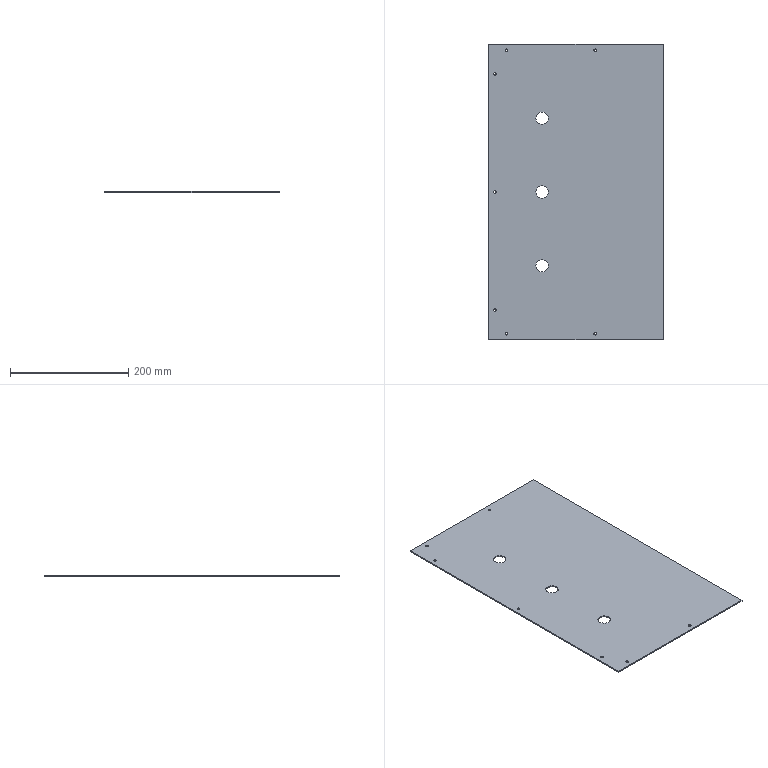Part | SolidWorks | features Extrusion 1, HoleWzd 1, ICE 1 | 1 solid | 26 faces | box 295 x 500 x 2 mm | volume 292699 mm3 | cylinder 20 | plane 6 | commonest cylinder face diameters 4.5 x14 21 x6
STEP:
#1=CARTESIAN_POINT('',(-68.,125.,0.));
#2=VERTEX_POINT('',#1);
#3=CARTESIAN_POINT('',(-47.,125.,0.));
#4=VERTEX_POINT('',#3);
#5=CARTESIAN_POINT('',(-57.5,125.,0.));
#6=DIRECTION('',(0.,0.,1.));
#7=DIRECTION('',(1.,0.,0.));
#8=AXIS2_PLACEMENT_3D('',#5,#6,#7);
#9=CIRCLE('',#8,10.5);
#10=EDGE_CURVE('',#2,#4,#9,.T.);
#11=ORIENTED_EDGE('',*,*,#10,.F.);
#12=CARTESIAN_POINT('',(-68.,125.,2.));
#13=VERTEX_POINT('',#12);
#14=CARTESIAN_POINT('',(-68.,125.,-8.));
#15=DIRECTION('',(0.,0.,1.));
#16=VECTOR('',#15,1000.);
#17=LINE('',#14,#16);
#18=EDGE_CURVE('',#2,#13,#17,.T.);
#19=ORIENTED_EDGE('',*,*,#18,.T.);
#20=CARTESIAN_POINT('',(-47.,125.,2.));
#21=VERTEX_POINT('',#20);
#22=CARTESIAN_POINT('',(-57.5,125.,2.));
#23=DIRECTION('',(0.,0.,1.));
#24=DIRECTION('',(1.,0.,0.));
#25=AXIS2_PLACEMENT_3D('',#22,#23,#24);
#26=CIRCLE('',#25,10.5);
#27=EDGE_CURVE('',#13,#21,#26,.T.);
#28=ORIENTED_EDGE('',*,*,#27,.T.);
#29=CARTESIAN_POINT('',(-47.,125.,-8.));
#30=DIRECTION('',(0.,0.,1.));
#31=VECTOR('',#30,1000.);
#32=LINE('',#29,#31);
#33=EDGE_CURVE('',#4,#21,#32,.T.);
#34=ORIENTED_EDGE('',*,*,#33,.F.);
#35=EDGE_LOOP('',(#11,#19,#28,#34));
#36=FACE_OUTER_BOUND('',#35,.T.);
#37=CARTESIAN_POINT('',(-57.5,125.,-8.));
#38=DIRECTION('',(0.,0.,1.));
#39=DIRECTION('',(1.,0.,0.));
#40=AXIS2_PLACEMENT_3D('',#37,#38,#39);
#41=CYLINDRICAL_SURFACE('',#40,10.5);
#42=ADVANCED_FACE('',(#36),#41,.F.);
#43=CARTESIAN_POINT('',(-68.,-125.,0.));
#44=VERTEX_POINT('',#43);
#45=CARTESIAN_POINT('',(-47.,-125.,0.));
#46=VERTEX_POINT('',#45);
#47=CARTESIAN_POINT('',(-57.5,-125.,0.));
#48=DIRECTION('',(0.,0.,1.));
#49=DIRECTION('',(1.,0.,0.));
#50=AXIS2_PLACEMENT_3D('',#47,#48,#49);
#51=CIRCLE('',#50,10.5);
#52=EDGE_CURVE('',#44,#46,#51,.T.);
#53=ORIENTED_EDGE('',*,*,#52,.F.);
#54=CARTESIAN_POINT('',(-68.,-125.,2.));
#55=VERTEX_POINT('',#54);
#56=CARTESIAN_POINT('',(-68.,-125.,-8.));
#57=DIRECTION('',(0.,0.,1.));
#58=VECTOR('',#57,1000.);
#59=LINE('',#56,#58);
#60=EDGE_CURVE('',#44,#55,#59,.T.);
#61=ORIENTED_EDGE('',*,*,#60,.T.);
#62=CARTESIAN_POINT('',(-47.,-125.,2.));
#63=VERTEX_POINT('',#62);
#64=CARTESIAN_POINT('',(-57.5,-125.,2.));
#65=DIRECTION('',(0.,0.,1.));
#66=DIRECTION('',(-1.,0.,0.));
#67=AXIS2_PLACEMENT_3D('',#64,#65,#66);
#68=CIRCLE('',#67,10.5);
#69=EDGE_CURVE('',#55,#63,#68,.T.);
#70=ORIENTED_EDGE('',*,*,#69,.T.);
#71=CARTESIAN_POINT('',(-47.,-125.,-8.));
#72=DIRECTION('',(0.,0.,1.));
#73=VECTOR('',#72,1000.);
#74=LINE('',#71,#73);
#75=EDGE_CURVE('',#46,#63,#74,.T.);
#76=ORIENTED_EDGE('',*,*,#75,.F.);
#77=EDGE_LOOP('',(#53,#61,#70,#76));
#78=FACE_OUTER_BOUND('',#77,.T.);
#79=CARTESIAN_POINT('',(-57.5,-125.,-8.));
#80=DIRECTION('',(0.,0.,1.));
#81=DIRECTION('',(1.,0.,0.));
#82=AXIS2_PLACEMENT_3D('',#79,#80,#81);
#83=CYLINDRICAL_SURFACE('',#82,10.5);
#84=ADVANCED_FACE('',(#78),#83,.F.);
#85=CARTESIAN_POINT('',(-68.,0.,0.));
#86=VERTEX_POINT('',#85);
#87=CARTESIAN_POINT('',(-47.,0.,0.));
#88=VERTEX_POINT('',#87);
#89=CARTESIAN_POINT('',(-57.5,0.,0.));
#90=DIRECTION('',(0.,0.,1.));
#91=DIRECTION('',(1.,0.,0.));
#92=AXIS2_PLACEMENT_3D('',#89,#90,#91);
#93=CIRCLE('',#92,10.5);
#94=EDGE_CURVE('',#86,#88,#93,.T.);
#95=ORIENTED_EDGE('',*,*,#94,.F.);
#96=CARTESIAN_POINT('',(-68.,0.,2.));
#97=VERTEX_POINT('',#96);
#98=CARTESIAN_POINT('',(-68.,0.,-8.));
#99=DIRECTION('',(0.,0.,1.));
#100=VECTOR('',#99,1000.);
#101=LINE('',#98,#100);
#102=EDGE_CURVE('',#86,#97,#101,.T.);
#103=ORIENTED_EDGE('',*,*,#102,.T.);
#104=CARTESIAN_POINT('',(-47.,0.,2.));
#105=VERTEX_POINT('',#104);
#106=CARTESIAN_POINT('',(-57.5,0.,2.));
#107=DIRECTION('',(0.,0.,1.));
#108=DIRECTION('',(1.,0.,0.));
#109=AXIS2_PLACEMENT_3D('',#106,#107,#108);
#110=CIRCLE('',#109,10.5);
#111=EDGE_CURVE('',#97,#105,#110,.T.);
#112=ORIENTED_EDGE('',*,*,#111,.T.);
#113=CARTESIAN_POINT('',(-47.,0.,-8.));
#114=DIRECTION('',(0.,0.,1.));
#115=VECTOR('',#114,1000.);
#116=LINE('',#113,#115);
#117=EDGE_CURVE('',#88,#105,#116,.T.);
#118=ORIENTED_EDGE('',*,*,#117,.F.);
#119=EDGE_LOOP('',(#95,#103,#112,#118));
#120=FACE_OUTER_BOUND('',#119,.T.);
#121=CARTESIAN_POINT('',(-57.5,0.,-8.));
#122=DIRECTION('',(0.,0.,1.));
#123=DIRECTION('',(1.,0.,0.));
#124=AXIS2_PLACEMENT_3D('',#121,#122,#123);
#125=CYLINDRICAL_SURFACE('',#124,10.5);
#126=ADVANCED_FACE('',(#120),#125,.F.);
#127=CARTESIAN_POINT('',(-139.75,0.,0.));
#128=VERTEX_POINT('',#127);
#129=CARTESIAN_POINT('',(-135.25,0.,0.));
#130=VERTEX_POINT('',#129);
#131=CARTESIAN_POINT('',(-137.5,0.,0.));
#132=DIRECTION('',(0.,0.,1.));
#133=DIRECTION('',(1.,0.,0.));
#134=AXIS2_PLACEMENT_3D('',#131,#132,#133);
#135=CIRCLE('',#134,2.25);
#136=EDGE_CURVE('',#128,#130,#135,.T.);
#137=ORIENTED_EDGE('',*,*,#136,.F.);
#138=CARTESIAN_POINT('',(-139.75,0.,2.));
#139=VERTEX_POINT('',#138);
#140=CARTESIAN_POINT('',(-139.75,0.,2.));
#141=DIRECTION('',(0.,0.,1.));
#142=VECTOR('',#141,1000.);
#143=LINE('',#140,#142);
#144=EDGE_CURVE('',#128,#139,#143,.T.);
#145=ORIENTED_EDGE('',*,*,#144,.T.);
#146=CARTESIAN_POINT('',(-135.25,0.,2.));
#147=VERTEX_POINT('',#146);
#148=CARTESIAN_POINT('',(-137.5,0.,2.));
#149=DIRECTION('',(0.,0.,1.));
#150=DIRECTION('',(1.,0.,0.));
#151=AXIS2_PLACEMENT_3D('',#148,#149,#150);
#152=CIRCLE('',#151,2.25);
#153=EDGE_CURVE('',#139,#147,#152,.T.);
#154=ORIENTED_EDGE('',*,*,#153,.T.);
#155=CARTESIAN_POINT('',(-135.25,0.,2.));
#156=DIRECTION('',(0.,0.,1.));
#157=VECTOR('',#156,1000.);
#158=LINE('',#155,#157);
#159=EDGE_CURVE('',#130,#147,#158,.T.);
#160=ORIENTED_EDGE('',*,*,#159,.F.);
#161=EDGE_LOOP('',(#137,#145,#154,#160));
#162=FACE_OUTER_BOUND('',#161,.T.);
#163=CARTESIAN_POINT('',(-137.5,0.,2.));
#164=DIRECTION('',(0.,0.,1.));
#165=DIRECTION('',(1.,0.,0.));
#166=AXIS2_PLACEMENT_3D('',#163,#164,#165);
#167=CYLINDRICAL_SURFACE('',#166,2.25);
#168=ADVANCED_FACE('',(#162),#167,.F.);
#169=CARTESIAN_POINT('',(-139.75,200.,0.));
#170=VERTEX_POINT('',#169);
#171=CARTESIAN_POINT('',(-135.25,200.,0.));
#172=VERTEX_POINT('',#171);
#173=CARTESIAN_POINT('',(-137.5,200.,0.));
#174=DIRECTION('',(0.,0.,1.));
#175=DIRECTION('',(1.,0.,0.));
#176=AXIS2_PLACEMENT_3D('',#173,#174,#175);
#177=CIRCLE('',#176,2.25);
#178=EDGE_CURVE('',#170,#172,#177,.T.);
#179=ORIENTED_EDGE('',*,*,#178,.F.);
#180=CARTESIAN_POINT('',(-139.75,200.,2.));
#181=VERTEX_POINT('',#180);
#182=CARTESIAN_POINT('',(-139.75,200.,2.));
#183=DIRECTION('',(0.,0.,1.));
#184=VECTOR('',#183,1000.);
#185=LINE('',#182,#184);
#186=EDGE_CURVE('',#170,#181,#185,.T.);
#187=ORIENTED_EDGE('',*,*,#186,.T.);
#188=CARTESIAN_POINT('',(-135.25,200.,2.));
#189=VERTEX_POINT('',#188);
#190=CARTESIAN_POINT('',(-137.5,200.,2.));
#191=DIRECTION('',(0.,0.,1.));
#192=DIRECTION('',(1.,0.,0.));
#193=AXIS2_PLACEMENT_3D('',#190,#191,#192);
#194=CIRCLE('',#193,2.25);
#195=EDGE_CURVE('',#181,#189,#194,.T.);
#196=ORIENTED_EDGE('',*,*,#195,.T.);
#197=CARTESIAN_POINT('',(-135.25,200.,2.));
#198=DIRECTION('',(0.,0.,1.));
#199=VECTOR('',#198,1000.);
#200=LINE('',#197,#199);
#201=EDGE_CURVE('',#172,#189,#200,.T.);
#202=ORIENTED_EDGE('',*,*,#201,.F.);
#203=EDGE_LOOP('',(#179,#187,#196,#202));
#204=FACE_OUTER_BOUND('',#203,.T.);
#205=CARTESIAN_POINT('',(-137.5,200.,2.));
#206=DIRECTION('',(0.,0.,1.));
#207=DIRECTION('',(1.,0.,0.));
#208=AXIS2_PLACEMENT_3D('',#205,#206,#207);
#209=CYLINDRICAL_SURFACE('',#208,2.25);
#210=ADVANCED_FACE('',(#204),#209,.F.);
#211=CARTESIAN_POINT('',(-139.75,-200.,0.));
#212=VERTEX_POINT('',#211);
#213=CARTESIAN_POINT('',(-135.25,-200.,0.));
#214=VERTEX_POINT('',#213);
#215=CARTESIAN_POINT('',(-137.5,-200.,0.));
#216=DIRECTION('',(0.,0.,1.));
#217=DIRECTION('',(1.,0.,0.));
#218=AXIS2_PLACEMENT_3D('',#215,#216,#217);
#219=CIRCLE('',#218,2.25);
#220=EDGE_CURVE('',#212,#214,#219,.T.);
#221=ORIENTED_EDGE('',*,*,#220,.F.);
#222=CARTESIAN_POINT('',(-139.75,-200.,2.));
#223=VERTEX_POINT('',#222);
#224=CARTESIAN_POINT('',(-139.75,-200.,2.));
#225=DIRECTION('',(0.,0.,1.));
#226=VECTOR('',#225,1000.);
#227=LINE('',#224,#226);
#228=EDGE_CURVE('',#212,#223,#227,.T.);
#229=ORIENTED_EDGE('',*,*,#228,.T.);
#230=CARTESIAN_POINT('',(-135.25,-200.,2.));
#231=VERTEX_POINT('',#230);
#232=CARTESIAN_POINT('',(-137.5,-200.,2.));
#233=DIRECTION('',(0.,0.,1.));
#234=DIRECTION('',(1.,0.,0.));
#235=AXIS2_PLACEMENT_3D('',#232,#233,#234);
#236=CIRCLE('',#235,2.25);
#237=EDGE_CURVE('',#223,#231,#236,.T.);
#238=ORIENTED_EDGE('',*,*,#237,.T.);
#239=CARTESIAN_POINT('',(-135.25,-200.,2.));
#240=DIRECTION('',(0.,0.,1.));
#241=VECTOR('',#240,1000.);
#242=LINE('',#239,#241);
#243=EDGE_CURVE('',#214,#231,#242,.T.);
#244=ORIENTED_EDGE('',*,*,#243,.F.);
#245=EDGE_LOOP('',(#221,#229,#238,#244));
#246=FACE_OUTER_BOUND('',#245,.T.);
#247=CARTESIAN_POINT('',(-137.5,-200.,2.));
#248=DIRECTION('',(0.,0.,1.));
#249=DIRECTION('',(1.,0.,0.));
#250=AXIS2_PLACEMENT_3D('',#247,#248,#249);
#251=CYLINDRICAL_SURFACE('',#250,2.25);
#252=ADVANCED_FACE('',(#246),#251,.F.);
#253=CARTESIAN_POINT('',(-119.75,240.,0.));
#254=VERTEX_POINT('',#253);
#255=CARTESIAN_POINT('',(-115.25,240.,0.));
#256=VERTEX_POINT('',#255);
#257=CARTESIAN_POINT('',(-117.5,240.,0.));
#258=DIRECTION('',(0.,0.,1.));
#259=DIRECTION('',(1.,0.,0.));
#260=AXIS2_PLACEMENT_3D('',#257,#258,#259);
#261=CIRCLE('',#260,2.25);
#262=EDGE_CURVE('',#254,#256,#261,.T.);
#263=ORIENTED_EDGE('',*,*,#262,.F.);
#264=CARTESIAN_POINT('',(-119.75,240.,2.));
#265=VERTEX_POINT('',#264);
#266=CARTESIAN_POINT('',(-119.75,240.,2.));
#267=DIRECTION('',(0.,0.,1.));
#268=VECTOR('',#267,1000.);
#269=LINE('',#266,#268);
#270=EDGE_CURVE('',#254,#265,#269,.T.);
#271=ORIENTED_EDGE('',*,*,#270,.T.);
#272=CARTESIAN_POINT('',(-115.25,240.,2.));
#273=VERTEX_POINT('',#272);
#274=CARTESIAN_POINT('',(-117.5,240.,2.));
#275=DIRECTION('',(0.,0.,1.));
#276=DIRECTION('',(1.,0.,0.));
#277=AXIS2_PLACEMENT_3D('',#274,#275,#276);
#278=CIRCLE('',#277,2.25);
#279=EDGE_CURVE('',#265,#273,#278,.T.);
#280=ORIENTED_EDGE('',*,*,#279,.T.);
#281=CARTESIAN_POINT('',(-115.25,240.,2.));
#282=DIRECTION('',(0.,0.,1.));
#283=VECTOR('',#282,1000.);
#284=LINE('',#281,#283);
#285=EDGE_CURVE('',#256,#273,#284,.T.);
#286=ORIENTED_EDGE('',*,*,#285,.F.);
#287=EDGE_LOOP('',(#263,#271,#280,#286));
#288=FACE_OUTER_BOUND('',#287,.T.);
#289=CARTESIAN_POINT('',(-117.5,240.,2.));
#290=DIRECTION('',(0.,0.,1.));
#291=DIRECTION('',(1.,0.,0.));
#292=AXIS2_PLACEMENT_3D('',#289,#290,#291);
#293=CYLINDRICAL_SURFACE('',#292,2.25);
#294=ADVANCED_FACE('',(#288),#293,.F.);
#295=CARTESIAN_POINT('',(30.25,240.,0.));
#296=VERTEX_POINT('',#295);
#297=CARTESIAN_POINT('',(34.75,240.,0.));
#298=VERTEX_POINT('',#297);
#299=CARTESIAN_POINT('',(32.5,240.,0.));
#300=DIRECTION('',(0.,0.,1.));
#301=DIRECTION('',(1.,0.,0.));
#302=AXIS2_PLACEMENT_3D('',#299,#300,#301);
#303=CIRCLE('',#302,2.25);
#304=EDGE_CURVE('',#296,#298,#303,.T.);
#305=ORIENTED_EDGE('',*,*,#304,.F.);
#306=CARTESIAN_POINT('',(30.25,240.,2.));
#307=VERTEX_POINT('',#306);
#308=CARTESIAN_POINT('',(30.25,240.,2.));
#309=DIRECTION('',(0.,0.,1.));
#310=VECTOR('',#309,1000.);
#311=LINE('',#308,#310);
#312=EDGE_CURVE('',#296,#307,#311,.T.);
#313=ORIENTED_EDGE('',*,*,#312,.T.);
#314=CARTESIAN_POINT('',(34.75,240.,2.));
#315=VERTEX_POINT('',#314);
#316=CARTESIAN_POINT('',(32.5,240.,2.));
#317=DIRECTION('',(0.,0.,1.));
#318=DIRECTION('',(1.,0.,0.));
#319=AXIS2_PLACEMENT_3D('',#316,#317,#318);
#320=CIRCLE('',#319,2.25);
#321=EDGE_CURVE('',#307,#315,#320,.T.);
#322=ORIENTED_EDGE('',*,*,#321,.T.);
#323=CARTESIAN_POINT('',(34.75,240.,2.));
#324=DIRECTION('',(0.,0.,1.));
#325=VECTOR('',#324,1000.);
#326=LINE('',#323,#325);
#327=EDGE_CURVE('',#298,#315,#326,.T.);
#328=ORIENTED_EDGE('',*,*,#327,.F.);
#329=EDGE_LOOP('',(#305,#313,#322,#328));
#330=FACE_OUTER_BOUND('',#329,.T.);
#331=CARTESIAN_POINT('',(32.5,240.,2.));
#332=DIRECTION('',(0.,0.,1.));
#333=DIRECTION('',(1.,0.,0.));
#334=AXIS2_PLACEMENT_3D('',#331,#332,#333);
#335=CYLINDRICAL_SURFACE('',#334,2.25);
#336=ADVANCED_FACE('',(#330),#335,.F.);
#337=CARTESIAN_POINT('',(30.25,-240.,0.));
#338=VERTEX_POINT('',#337);
#339=CARTESIAN_POINT('',(34.75,-240.,0.));
#340=VERTEX_POINT('',#339);
#341=CARTESIAN_POINT('',(32.5,-240.,0.));
#342=DIRECTION('',(0.,0.,1.));
#343=DIRECTION('',(1.,0.,0.));
#344=AXIS2_PLACEMENT_3D('',#341,#342,#343);
#345=CIRCLE('',#344,2.25);
#346=EDGE_CURVE('',#338,#340,#345,.T.);
#347=ORIENTED_EDGE('',*,*,#346,.F.);
#348=CARTESIAN_POINT('',(30.25,-240.,2.));
#349=VERTEX_POINT('',#348);
#350=CARTESIAN_POINT('',(30.25,-240.,2.));
#351=DIRECTION('',(0.,0.,1.));
#352=VECTOR('',#351,1000.);
#353=LINE('',#350,#352);
#354=EDGE_CURVE('',#338,#349,#353,.T.);
#355=ORIENTED_EDGE('',*,*,#354,.T.);
#356=CARTESIAN_POINT('',(34.75,-240.,2.));
#357=VERTEX_POINT('',#356);
#358=CARTESIAN_POINT('',(32.5,-240.,2.));
#359=DIRECTION('',(0.,0.,1.));
#360=DIRECTION('',(1.,0.,0.));
#361=AXIS2_PLACEMENT_3D('',#358,#359,#360);
#362=CIRCLE('',#361,2.25);
#363=EDGE_CURVE('',#349,#357,#362,.T.);
#364=ORIENTED_EDGE('',*,*,#363,.T.);
#365=CARTESIAN_POINT('',(34.75,-240.,2.));
#366=DIRECTION('',(0.,0.,1.));
#367=VECTOR('',#366,1000.);
#368=LINE('',#365,#367);
#369=EDGE_CURVE('',#340,#357,#368,.T.);
#370=ORIENTED_EDGE('',*,*,#369,.F.);
#371=EDGE_LOOP('',(#347,#355,#364,#370));
#372=FACE_OUTER_BOUND('',#371,.T.);
#373=CARTESIAN_POINT('',(32.5,-240.,2.));
#374=DIRECTION('',(0.,0.,1.));
#375=DIRECTION('',(1.,0.,0.));
#376=AXIS2_PLACEMENT_3D('',#373,#374,#375);
#377=CYLINDRICAL_SURFACE('',#376,2.25);
#378=ADVANCED_FACE('',(#372),#377,.F.);
#379=CARTESIAN_POINT('',(-119.75,-240.,0.));
#380=VERTEX_POINT('',#379);
#381=CARTESIAN_POINT('',(-115.25,-240.,0.));
#382=VERTEX_POINT('',#381);
#383=CARTESIAN_POINT('',(-117.5,-240.,0.));
#384=DIRECTION('',(0.,0.,1.));
#385=DIRECTION('',(1.,0.,0.));
#386=AXIS2_PLACEMENT_3D('',#383,#384,#385);
#387=CIRCLE('',#386,2.25);
#388=EDGE_CURVE('',#380,#382,#387,.T.);
#389=ORIENTED_EDGE('',*,*,#388,.F.);
#390=CARTESIAN_POINT('',(-119.75,-240.,2.));
#391=VERTEX_POINT('',#390);
#392=CARTESIAN_POINT('',(-119.75,-240.,2.));
#393=DIRECTION('',(0.,0.,1.));
#394=VECTOR('',#393,1000.);
#395=LINE('',#392,#394);
#396=EDGE_CURVE('',#380,#391,#395,.T.);
#397=ORIENTED_EDGE('',*,*,#396,.T.);
#398=CARTESIAN_POINT('',(-115.25,-240.,2.));
#399=VERTEX_POINT('',#398);
#400=CARTESIAN_POINT('',(-117.5,-240.,2.));
#401=DIRECTION('',(0.,0.,1.));
#402=DIRECTION('',(1.,0.,0.));
#403=AXIS2_PLACEMENT_3D('',#400,#401,#402);
#404=CIRCLE('',#403,2.25);
#405=EDGE_CURVE('',#391,#399,#404,.T.);
#406=ORIENTED_EDGE('',*,*,#405,.T.);
#407=CARTESIAN_POINT('',(-115.25,-240.,2.));
#408=DIRECTION('',(0.,0.,1.));
#409=VECTOR('',#408,1000.);
#410=LINE('',#407,#409);
#411=EDGE_CURVE('',#382,#399,#410,.T.);
#412=ORIENTED_EDGE('',*,*,#411,.F.);
#413=EDGE_LOOP('',(#389,#397,#406,#412));
#414=FACE_OUTER_BOUND('',#413,.T.);
#415=CARTESIAN_POINT('',(-117.5,-240.,2.));
#416=DIRECTION('',(0.,0.,1.));
#417=DIRECTION('',(1.,0.,0.));
#418=AXIS2_PLACEMENT_3D('',#415,#416,#417);
#419=CYLINDRICAL_SURFACE('',#418,2.25);
#420=ADVANCED_FACE('',(#414),#419,.F.);
#421=CARTESIAN_POINT('',(147.5,-250.,0.));
#422=VERTEX_POINT('',#421);
#423=CARTESIAN_POINT('',(147.5,250.,0.));
#424=VERTEX_POINT('',#423);
#425=CARTESIAN_POINT('',(147.5,250.,0.));
#426=DIRECTION('',(0.,1.,0.));
#427=VECTOR('',#426,1000.);
#428=LINE('',#425,#427);
#429=EDGE_CURVE('',#422,#424,#428,.T.);
#430=ORIENTED_EDGE('',*,*,#429,.T.);
#431=CARTESIAN_POINT('',(147.5,250.,2.));
#432=VERTEX_POINT('',#431);
#433=CARTESIAN_POINT('',(147.5,250.,2.));
#434=DIRECTION('',(0.,0.,-1.));
#435=VECTOR('',#434,1000.);
#436=LINE('',#433,#435);
#437=EDGE_CURVE('',#432,#424,#436,.T.);
#438=ORIENTED_EDGE('',*,*,#437,.F.);
#439=CARTESIAN_POINT('',(147.5,-250.,2.));
#440=VERTEX_POINT('',#439);
#441=CARTESIAN_POINT('',(147.5,250.,2.));
#442=DIRECTION('',(0.,1.,0.));
#443=VECTOR('',#442,1000.);
#444=LINE('',#441,#443);
#445=EDGE_CURVE('',#440,#432,#444,.T.);
#446=ORIENTED_EDGE('',*,*,#445,.F.);
#447=CARTESIAN_POINT('',(147.5,-250.,2.));
#448=DIRECTION('',(0.,0.,-1.));
#449=VECTOR('',#448,1000.);
#450=LINE('',#447,#449);
#451=EDGE_CURVE('',#440,#422,#450,.T.);
#452=ORIENTED_EDGE('',*,*,#451,.T.);
#453=EDGE_LOOP('',(#430,#438,#446,#452));
#454=FACE_OUTER_BOUND('',#453,.T.);
#455=CARTESIAN_POINT('',(147.5,250.,2.));
#456=DIRECTION('',(-1.,0.,0.));
#457=DIRECTION('',(0.,0.,1.));
#458=AXIS2_PLACEMENT_3D('',#455,#456,#457);
#459=PLANE('',#458);
#460=ADVANCED_FACE('',(#454),#459,.F.);
#461=CARTESIAN_POINT('',(-147.5,250.,0.));
#462=VERTEX_POINT('',#461);
#463=CARTESIAN_POINT('',(-147.5,250.,0.));
#464=DIRECTION('',(-1.,0.,0.));
#465=VECTOR('',#464,1000.);
#466=LINE('',#463,#465);
#467=EDGE_CURVE('',#424,#462,#466,.T.);
#468=ORIENTED_EDGE('',*,*,#467,.T.);
#469=CARTESIAN_POINT('',(-147.5,250.,2.));
#470=VERTEX_POINT('',#469);
#471=CARTESIAN_POINT('',(-147.5,250.,2.));
#472=DIRECTION('',(0.,0.,-1.));
#473=VECTOR('',#472,1000.);
#474=LINE('',#471,#473);
#475=EDGE_CURVE('',#470,#462,#474,.T.);
#476=ORIENTED_EDGE('',*,*,#475,.F.);
#477=CARTESIAN_POINT('',(-147.5,250.,2.));
#478=DIRECTION('',(-1.,0.,0.));
#479=VECTOR('',#478,1000.);
#480=LINE('',#477,#479);
#481=EDGE_CURVE('',#432,#470,#480,.T.);
#482=ORIENTED_EDGE('',*,*,#481,.F.);
#483=ORIENTED_EDGE('',*,*,#437,.T.);
#484=EDGE_LOOP('',(#468,#476,#482,#483));
#485=FACE_OUTER_BOUND('',#484,.T.);
#486=CARTESIAN_POINT('',(-147.5,250.,2.));
#487=DIRECTION('',(0.,-1.,0.));
#488=DIRECTION('',(0.,0.,-1.));
#489=AXIS2_PLACEMENT_3D('',#486,#487,#488);
#490=PLANE('',#489);
#491=ADVANCED_FACE('',(#485),#490,.F.);
#492=CARTESIAN_POINT('',(-147.5,-250.,0.));
#493=VERTEX_POINT('',#492);
#494=CARTESIAN_POINT('',(-147.5,250.,0.));
#495=DIRECTION('',(0.,-1.,0.));
#496=VECTOR('',#495,1000.);
#497=LINE('',#494,#496);
#498=EDGE_CURVE('',#462,#493,#497,.T.);
#499=ORIENTED_EDGE('',*,*,#498,.T.);
#500=CARTESIAN_POINT('',(-147.5,-250.,2.));
#501=VERTEX_POINT('',#500);
#502=CARTESIAN_POINT('',(-147.5,-250.,2.));
#503=DIRECTION('',(0.,0.,-1.));
#504=VECTOR('',#503,1000.);
#505=LINE('',#502,#504);
#506=EDGE_CURVE('',#501,#493,#505,.T.);
#507=ORIENTED_EDGE('',*,*,#506,.F.);
#508=CARTESIAN_POINT('',(-147.5,250.,2.));
#509=DIRECTION('',(0.,-1.,0.));
#510=VECTOR('',#509,1000.);
#511=LINE('',#508,#510);
#512=EDGE_CURVE('',#470,#501,#511,.T.);
#513=ORIENTED_EDGE('',*,*,#512,.F.);
#514=ORIENTED_EDGE('',*,*,#475,.T.);
#515=EDGE_LOOP('',(#499,#507,#513,#514));
#516=FACE_OUTER_BOUND('',#515,.T.);
#517=CARTESIAN_POINT('',(-147.5,250.,2.));
#518=DIRECTION('',(1.,0.,0.));
#519=DIRECTION('',(0.,0.,-1.));
#520=AXIS2_PLACEMENT_3D('',#517,#518,#519);
#521=PLANE('',#520);
#522=ADVANCED_FACE('',(#516),#521,.F.);
#523=CARTESIAN_POINT('',(-147.5,-250.,0.));
#524=DIRECTION('',(1.,0.,0.));
#525=VECTOR('',#524,1000.);
#526=LINE('',#523,#525);
#527=EDGE_CURVE('',#493,#422,#526,.T.);
#528=ORIENTED_EDGE('',*,*,#527,.T.);
#529=ORIENTED_EDGE('',*,*,#451,.F.);
#530=CARTESIAN_POINT('',(-147.5,-250.,2.));
#531=DIRECTION('',(1.,0.,0.));
#532=VECTOR('',#531,1000.);
#533=LINE('',#530,#532);
#534=EDGE_CURVE('',#501,#440,#533,.T.);
#535=ORIENTED_EDGE('',*,*,#534,.F.);
#536=ORIENTED_EDGE('',*,*,#506,.T.);
#537=EDGE_LOOP('',(#528,#529,#535,#536));
#538=FACE_OUTER_BOUND('',#537,.T.);
#539=CARTESIAN_POINT('',(-147.5,-250.,2.));
#540=DIRECTION('',(0.,1.,0.));
#541=DIRECTION('',(0.,0.,1.));
#542=AXIS2_PLACEMENT_3D('',#539,#540,#541);
#543=PLANE('',#542);
#544=ADVANCED_FACE('',(#538),#543,.F.);
#545=CARTESIAN_POINT('',(-57.5,125.,2.));
#546=DIRECTION('',(0.,0.,1.));
#547=DIRECTION('',(1.,0.,0.));
#548=AXIS2_PLACEMENT_3D('',#545,#546,#547);
#549=CIRCLE('',#548,10.5);
#550=EDGE_CURVE('',#21,#13,#549,.T.);
#551=ORIENTED_EDGE('',*,*,#550,.F.);
#552=ORIENTED_EDGE('',*,*,#27,.F.);
#553=EDGE_LOOP('',(#551,#552));
#554=FACE_BOUND('',#553,.T.);
#555=CARTESIAN_POINT('',(-57.5,-125.,2.));
#556=DIRECTION('',(0.,0.,1.));
#557=DIRECTION('',(-1.,0.,0.));
#558=AXIS2_PLACEMENT_3D('',#555,#556,#557);
#559=CIRCLE('',#558,10.5);
#560=EDGE_CURVE('',#63,#55,#559,.T.);
#561=ORIENTED_EDGE('',*,*,#560,.F.);
#562=ORIENTED_EDGE('',*,*,#69,.F.);
#563=EDGE_LOOP('',(#561,#562));
#564=FACE_BOUND('',#563,.T.);
#565=CARTESIAN_POINT('',(-57.5,0.,2.));
#566=DIRECTION('',(0.,0.,1.));
#567=DIRECTION('',(1.,0.,0.));
#568=AXIS2_PLACEMENT_3D('',#565,#566,#567);
#569=CIRCLE('',#568,10.5);
#570=EDGE_CURVE('',#105,#97,#569,.T.);
#571=ORIENTED_EDGE('',*,*,#570,.F.);
#572=ORIENTED_EDGE('',*,*,#111,.F.);
#573=EDGE_LOOP('',(#571,#572));
#574=FACE_BOUND('',#573,.T.);
#575=CARTESIAN_POINT('',(-137.5,0.,2.));
#576=DIRECTION('',(0.,0.,1.));
#577=DIRECTION('',(1.,0.,0.));
#578=AXIS2_PLACEMENT_3D('',#575,#576,#577);
#579=CIRCLE('',#578,2.25);
#580=EDGE_CURVE('',#147,#139,#579,.T.);
#581=ORIENTED_EDGE('',*,*,#580,.F.);
#582=ORIENTED_EDGE('',*,*,#153,.F.);
#583=EDGE_LOOP('',(#581,#582));
#584=FACE_BOUND('',#583,.T.);
#585=CARTESIAN_POINT('',(-137.5,200.,2.));
#586=DIRECTION('',(0.,0.,1.));
#587=DIRECTION('',(1.,0.,0.));
#588=AXIS2_PLACEMENT_3D('',#585,#586,#587);
#589=CIRCLE('',#588,2.25);
#590=EDGE_CURVE('',#189,#181,#589,.T.);
#591=ORIENTED_EDGE('',*,*,#590,.F.);
#592=ORIENTED_EDGE('',*,*,#195,.F.);
#593=EDGE_LOOP('',(#591,#592));
#594=FACE_BOUND('',#593,.T.);
#595=CARTESIAN_POINT('',(-137.5,-200.,2.));
#596=DIRECTION('',(0.,0.,1.));
#597=DIRECTION('',(1.,0.,0.));
#598=AXIS2_PLACEMENT_3D('',#595,#596,#597);
#599=CIRCLE('',#598,2.25);
#600=EDGE_CURVE('',#231,#223,#599,.T.);
#601=ORIENTED_EDGE('',*,*,#600,.F.);
#602=ORIENTED_EDGE('',*,*,#237,.F.);
#603=EDGE_LOOP('',(#601,#602));
#604=FACE_BOUND('',#603,.T.);
#605=CARTESIAN_POINT('',(-117.5,240.,2.));
#606=DIRECTION('',(0.,0.,1.));
#607=DIRECTION('',(1.,0.,0.));
#608=AXIS2_PLACEMENT_3D('',#605,#606,#607);
#609=CIRCLE('',#608,2.25);
#610=EDGE_CURVE('',#273,#265,#609,.T.);
#611=ORIENTED_EDGE('',*,*,#610,.F.);
#612=ORIENTED_EDGE('',*,*,#279,.F.);
#613=EDGE_LOOP('',(#611,#612));
#614=FACE_BOUND('',#613,.T.);
#615=CARTESIAN_POINT('',(32.5,240.,2.));
#616=DIRECTION('',(0.,0.,1.));
#617=DIRECTION('',(1.,0.,0.));
#618=AXIS2_PLACEMENT_3D('',#615,#616,#617);
#619=CIRCLE('',#618,2.25);
#620=EDGE_CURVE('',#315,#307,#619,.T.);
#621=ORIENTED_EDGE('',*,*,#620,.F.);
#622=ORIENTED_EDGE('',*,*,#321,.F.);
#623=EDGE_LOOP('',(#621,#622));
#624=FACE_BOUND('',#623,.T.);
#625=CARTESIAN_POINT('',(32.5,-240.,2.));
#626=DIRECTION('',(0.,0.,1.));
#627=DIRECTION('',(1.,0.,0.));
#628=AXIS2_PLACEMENT_3D('',#625,#626,#627);
#629=CIRCLE('',#628,2.25);
#630=EDGE_CURVE('',#357,#349,#629,.T.);
#631=ORIENTED_EDGE('',*,*,#630,.F.);
#632=ORIENTED_EDGE('',*,*,#363,.F.);
#633=EDGE_LOOP('',(#631,#632));
#634=FACE_BOUND('',#633,.T.);
#635=CARTESIAN_POINT('',(-117.5,-240.,2.));
#636=DIRECTION('',(0.,0.,1.));
#637=DIRECTION('',(1.,0.,0.));
#638=AXIS2_PLACEMENT_3D('',#635,#636,#637);
#639=CIRCLE('',#638,2.25);
#640=EDGE_CURVE('',#399,#391,#639,.T.);
#641=ORIENTED_EDGE('',*,*,#640,.F.);
#642=ORIENTED_EDGE('',*,*,#405,.F.);
#643=EDGE_LOOP('',(#641,#642));
#644=FACE_BOUND('',#643,.T.);
#645=ORIENTED_EDGE('',*,*,#445,.T.);
#646=ORIENTED_EDGE('',*,*,#481,.T.);
#647=ORIENTED_EDGE('',*,*,#512,.T.);
#648=ORIENTED_EDGE('',*,*,#534,.T.);
#649=EDGE_LOOP('',(#645,#646,#647,#648));
#650=FACE_OUTER_BOUND('',#649,.T.);
#651=CARTESIAN_POINT('',(0.,0.,2.));
#652=DIRECTION('',(0.,0.,1.));
#653=DIRECTION('',(1.,0.,0.));
#654=AXIS2_PLACEMENT_3D('',#651,#652,#653);
#655=PLANE('',#654);
#656=ADVANCED_FACE('',(#554,#564,#574,#584,#594,#604,#614,#624,#634,#644,#650),#655,.T.);
#657=CARTESIAN_POINT('',(-57.5,125.,0.));
#658=DIRECTION('',(0.,0.,1.));
#659=DIRECTION('',(1.,0.,0.));
#660=AXIS2_PLACEMENT_3D('',#657,#658,#659);
#661=CIRCLE('',#660,10.5);
#662=EDGE_CURVE('',#4,#2,#661,.T.);
#663=ORIENTED_EDGE('',*,*,#662,.T.);
#664=ORIENTED_EDGE('',*,*,#10,.T.);
#665=EDGE_LOOP('',(#663,#664));
#666=FACE_BOUND('',#665,.T.);
#667=CARTESIAN_POINT('',(-57.5,-125.,0.));
#668=DIRECTION('',(0.,0.,1.));
#669=DIRECTION('',(1.,0.,0.));
#670=AXIS2_PLACEMENT_3D('',#667,#668,#669);
#671=CIRCLE('',#670,10.5);
#672=EDGE_CURVE('',#46,#44,#671,.T.);
#673=ORIENTED_EDGE('',*,*,#672,.T.);
#674=ORIENTED_EDGE('',*,*,#52,.T.);
#675=EDGE_LOOP('',(#673,#674));
#676=FACE_BOUND('',#675,.T.);
#677=CARTESIAN_POINT('',(-57.5,0.,0.));
#678=DIRECTION('',(0.,0.,1.));
#679=DIRECTION('',(1.,0.,0.));
#680=AXIS2_PLACEMENT_3D('',#677,#678,#679);
#681=CIRCLE('',#680,10.5);
#682=EDGE_CURVE('',#88,#86,#681,.T.);
#683=ORIENTED_EDGE('',*,*,#682,.T.);
#684=ORIENTED_EDGE('',*,*,#94,.T.);
#685=EDGE_LOOP('',(#683,#684));
#686=FACE_BOUND('',#685,.T.);
#687=CARTESIAN_POINT('',(-137.5,0.,0.));
#688=DIRECTION('',(0.,0.,1.));
#689=DIRECTION('',(1.,0.,0.));
#690=AXIS2_PLACEMENT_3D('',#687,#688,#689);
#691=CIRCLE('',#690,2.25);
#692=EDGE_CURVE('',#130,#128,#691,.T.);
#693=ORIENTED_EDGE('',*,*,#692,.T.);
#694=ORIENTED_EDGE('',*,*,#136,.T.);
#695=EDGE_LOOP('',(#693,#694));
#696=FACE_BOUND('',#695,.T.);
#697=CARTESIAN_POINT('',(-137.5,200.,0.));
#698=DIRECTION('',(0.,0.,1.));
#699=DIRECTION('',(1.,0.,0.));
#700=AXIS2_PLACEMENT_3D('',#697,#698,#699);
#701=CIRCLE('',#700,2.25);
#702=EDGE_CURVE('',#172,#170,#701,.T.);
#703=ORIENTED_EDGE('',*,*,#702,.T.);
#704=ORIENTED_EDGE('',*,*,#178,.T.);
#705=EDGE_LOOP('',(#703,#704));
#706=FACE_BOUND('',#705,.T.);
#707=CARTESIAN_POINT('',(-137.5,-200.,0.));
#708=DIRECTION('',(0.,0.,1.));
#709=DIRECTION('',(1.,0.,0.));
#710=AXIS2_PLACEMENT_3D('',#707,#708,#709);
#711=CIRCLE('',#710,2.25);
#712=EDGE_CURVE('',#214,#212,#711,.T.);
#713=ORIENTED_EDGE('',*,*,#712,.T.);
#714=ORIENTED_EDGE('',*,*,#220,.T.);
#715=EDGE_LOOP('',(#713,#714));
#716=FACE_BOUND('',#715,.T.);
#717=CARTESIAN_POINT('',(-117.5,240.,0.));
#718=DIRECTION('',(0.,0.,1.));
#719=DIRECTION('',(1.,0.,0.));
#720=AXIS2_PLACEMENT_3D('',#717,#718,#719);
#721=CIRCLE('',#720,2.25);
#722=EDGE_CURVE('',#256,#254,#721,.T.);
#723=ORIENTED_EDGE('',*,*,#722,.T.);
#724=ORIENTED_EDGE('',*,*,#262,.T.);
#725=EDGE_LOOP('',(#723,#724));
#726=FACE_BOUND('',#725,.T.);
#727=CARTESIAN_POINT('',(32.5,240.,0.));
#728=DIRECTION('',(0.,0.,1.));
#729=DIRECTION('',(1.,0.,0.));
#730=AXIS2_PLACEMENT_3D('',#727,#728,#729);
#731=CIRCLE('',#730,2.25);
#732=EDGE_CURVE('',#298,#296,#731,.T.);
#733=ORIENTED_EDGE('',*,*,#732,.T.);
#734=ORIENTED_EDGE('',*,*,#304,.T.);
#735=EDGE_LOOP('',(#733,#734));
#736=FACE_BOUND('',#735,.T.);
#737=CARTESIAN_POINT('',(32.5,-240.,0.));
#738=DIRECTION('',(0.,0.,1.));
#739=DIRECTION('',(1.,0.,0.));
#740=AXIS2_PLACEMENT_3D('',#737,#738,#739);
#741=CIRCLE('',#740,2.25);
#742=EDGE_CURVE('',#340,#338,#741,.T.);
#743=ORIENTED_EDGE('',*,*,#742,.T.);
#744=ORIENTED_EDGE('',*,*,#346,.T.);
#745=EDGE_LOOP('',(#743,#744));
#746=FACE_BOUND('',#745,.T.);
#747=CARTESIAN_POINT('',(-117.5,-240.,0.));
#748=DIRECTION('',(0.,0.,1.));
#749=DIRECTION('',(1.,0.,0.));
#750=AXIS2_PLACEMENT_3D('',#747,#748,#749);
#751=CIRCLE('',#750,2.25);
#752=EDGE_CURVE('',#382,#380,#751,.T.);
#753=ORIENTED_EDGE('',*,*,#752,.T.);
#754=ORIENTED_EDGE('',*,*,#388,.T.);
#755=EDGE_LOOP('',(#753,#754));
#756=FACE_BOUND('',#755,.T.);
#757=ORIENTED_EDGE('',*,*,#429,.F.);
#758=ORIENTED_EDGE('',*,*,#527,.F.);
#759=ORIENTED_EDGE('',*,*,#498,.F.);
#760=ORIENTED_EDGE('',*,*,#467,.F.);
#761=EDGE_LOOP('',(#757,#758,#759,#760));
#762=FACE_OUTER_BOUND('',#761,.T.);
#763=CARTESIAN_POINT('',(0.,0.,0.));
#764=DIRECTION('',(0.,0.,1.));
#765=DIRECTION('',(1.,0.,0.));
#766=AXIS2_PLACEMENT_3D('',#763,#764,#765);
#767=PLANE('',#766);
#768=ADVANCED_FACE('',(#666,#676,#686,#696,#706,#716,#726,#736,#746,#756,#762),#767,.F.);
#769=ORIENTED_EDGE('',*,*,#396,.F.);
#770=ORIENTED_EDGE('',*,*,#752,.F.);
#771=ORIENTED_EDGE('',*,*,#411,.T.);
#772=ORIENTED_EDGE('',*,*,#640,.T.);
#773=EDGE_LOOP('',(#769,#770,#771,#772));
#774=FACE_OUTER_BOUND('',#773,.T.);
#775=CARTESIAN_POINT('',(-117.5,-240.,2.));
#776=DIRECTION('',(0.,0.,1.));
#777=DIRECTION('',(1.,0.,0.));
#778=AXIS2_PLACEMENT_3D('',#775,#776,#777);
#779=CYLINDRICAL_SURFACE('',#778,2.25);
#780=ADVANCED_FACE('',(#774),#779,.F.);
#781=ORIENTED_EDGE('',*,*,#354,.F.);
#782=ORIENTED_EDGE('',*,*,#742,.F.);
#783=ORIENTED_EDGE('',*,*,#369,.T.);
#784=ORIENTED_EDGE('',*,*,#630,.T.);
#785=EDGE_LOOP('',(#781,#782,#783,#784));
#786=FACE_OUTER_BOUND('',#785,.T.);
#787=CARTESIAN_POINT('',(32.5,-240.,2.));
#788=DIRECTION('',(0.,0.,1.));
#789=DIRECTION('',(1.,0.,0.));
#790=AXIS2_PLACEMENT_3D('',#787,#788,#789);
#791=CYLINDRICAL_SURFACE('',#790,2.25);
#792=ADVANCED_FACE('',(#786),#791,.F.);
#793=ORIENTED_EDGE('',*,*,#312,.F.);
#794=ORIENTED_EDGE('',*,*,#732,.F.);
#795=ORIENTED_EDGE('',*,*,#327,.T.);
#796=ORIENTED_EDGE('',*,*,#620,.T.);
#797=EDGE_LOOP('',(#793,#794,#795,#796));
#798=FACE_OUTER_BOUND('',#797,.T.);
#799=CARTESIAN_POINT('',(32.5,240.,2.));
#800=DIRECTION('',(0.,0.,1.));
#801=DIRECTION('',(1.,0.,0.));
#802=AXIS2_PLACEMENT_3D('',#799,#800,#801);
#803=CYLINDRICAL_SURFACE('',#802,2.25);
#804=ADVANCED_FACE('',(#798),#803,.F.);
#805=ORIENTED_EDGE('',*,*,#270,.F.);
#806=ORIENTED_EDGE('',*,*,#722,.F.);
#807=ORIENTED_EDGE('',*,*,#285,.T.);
#808=ORIENTED_EDGE('',*,*,#610,.T.);
#809=EDGE_LOOP('',(#805,#806,#807,#808));
#810=FACE_OUTER_BOUND('',#809,.T.);
#811=CARTESIAN_POINT('',(-117.5,240.,2.));
#812=DIRECTION('',(0.,0.,1.));
#813=DIRECTION('',(1.,0.,0.));
#814=AXIS2_PLACEMENT_3D('',#811,#812,#813);
#815=CYLINDRICAL_SURFACE('',#814,2.25);
#816=ADVANCED_FACE('',(#810),#815,.F.);
#817=ORIENTED_EDGE('',*,*,#228,.F.);
#818=ORIENTED_EDGE('',*,*,#712,.F.);
#819=ORIENTED_EDGE('',*,*,#243,.T.);
#820=ORIENTED_EDGE('',*,*,#600,.T.);
#821=EDGE_LOOP('',(#817,#818,#819,#820));
#822=FACE_OUTER_BOUND('',#821,.T.);
#823=CARTESIAN_POINT('',(-137.5,-200.,2.));
#824=DIRECTION('',(0.,0.,1.));
#825=DIRECTION('',(1.,0.,0.));
#826=AXIS2_PLACEMENT_3D('',#823,#824,#825);
#827=CYLINDRICAL_SURFACE('',#826,2.25);
#828=ADVANCED_FACE('',(#822),#827,.F.);
#829=ORIENTED_EDGE('',*,*,#186,.F.);
#830=ORIENTED_EDGE('',*,*,#702,.F.);
#831=ORIENTED_EDGE('',*,*,#201,.T.);
#832=ORIENTED_EDGE('',*,*,#590,.T.);
#833=EDGE_LOOP('',(#829,#830,#831,#832));
#834=FACE_OUTER_BOUND('',#833,.T.);
#835=CARTESIAN_POINT('',(-137.5,200.,2.));
#836=DIRECTION('',(0.,0.,1.));
#837=DIRECTION('',(1.,0.,0.));
#838=AXIS2_PLACEMENT_3D('',#835,#836,#837);
#839=CYLINDRICAL_SURFACE('',#838,2.25);
#840=ADVANCED_FACE('',(#834),#839,.F.);
#841=ORIENTED_EDGE('',*,*,#144,.F.);
#842=ORIENTED_EDGE('',*,*,#692,.F.);
#843=ORIENTED_EDGE('',*,*,#159,.T.);
#844=ORIENTED_EDGE('',*,*,#580,.T.);
#845=EDGE_LOOP('',(#841,#842,#843,#844));
#846=FACE_OUTER_BOUND('',#845,.T.);
#847=CARTESIAN_POINT('',(-137.5,0.,2.));
#848=DIRECTION('',(0.,0.,1.));
#849=DIRECTION('',(1.,0.,0.));
#850=AXIS2_PLACEMENT_3D('',#847,#848,#849);
#851=CYLINDRICAL_SURFACE('',#850,2.25);
#852=ADVANCED_FACE('',(#846),#851,.F.);
#853=ORIENTED_EDGE('',*,*,#102,.F.);
#854=ORIENTED_EDGE('',*,*,#682,.F.);
#855=ORIENTED_EDGE('',*,*,#117,.T.);
#856=ORIENTED_EDGE('',*,*,#570,.T.);
#857=EDGE_LOOP('',(#853,#854,#855,#856));
#858=FACE_OUTER_BOUND('',#857,.T.);
#859=CARTESIAN_POINT('',(-57.5,0.,-8.));
#860=DIRECTION('',(0.,0.,1.));
#861=DIRECTION('',(1.,0.,0.));
#862=AXIS2_PLACEMENT_3D('',#859,#860,#861);
#863=CYLINDRICAL_SURFACE('',#862,10.5);
#864=ADVANCED_FACE('',(#858),#863,.F.);
#865=ORIENTED_EDGE('',*,*,#60,.F.);
#866=ORIENTED_EDGE('',*,*,#672,.F.);
#867=ORIENTED_EDGE('',*,*,#75,.T.);
#868=ORIENTED_EDGE('',*,*,#560,.T.);
#869=EDGE_LOOP('',(#865,#866,#867,#868));
#870=FACE_OUTER_BOUND('',#869,.T.);
#871=CARTESIAN_POINT('',(-57.5,-125.,-8.));
#872=DIRECTION('',(0.,0.,1.));
#873=DIRECTION('',(1.,0.,0.));
#874=AXIS2_PLACEMENT_3D('',#871,#872,#873);
#875=CYLINDRICAL_SURFACE('',#874,10.5);
#876=ADVANCED_FACE('',(#870),#875,.F.);
#877=ORIENTED_EDGE('',*,*,#18,.F.);
#878=ORIENTED_EDGE('',*,*,#662,.F.);
#879=ORIENTED_EDGE('',*,*,#33,.T.);
#880=ORIENTED_EDGE('',*,*,#550,.T.);
#881=EDGE_LOOP('',(#877,#878,#879,#880));
#882=FACE_OUTER_BOUND('',#881,.T.);
#883=CARTESIAN_POINT('',(-57.5,125.,-8.));
#884=DIRECTION('',(0.,0.,1.));
#885=DIRECTION('',(1.,0.,0.));
#886=AXIS2_PLACEMENT_3D('',#883,#884,#885);
#887=CYLINDRICAL_SURFACE('',#886,10.5);
#888=ADVANCED_FACE('',(#882),#887,.F.);
#889=CLOSED_SHELL('',(#42,#84,#126,#168,#210,#252,#294,#336,#378,#420,#460,#491,#522,#544,#656,#768,#780,#792,#804,#816,#828,#840,#852,#864,#876,#888));
#890=MANIFOLD_SOLID_BREP('',#889);
#891=CARTESIAN_POINT('',(0.,0.,0.));
#892=DIRECTION('',(0.,0.,1.));
#893=DIRECTION('',(1.,0.,0.));
#894=AXIS2_PLACEMENT_3D('',#891,#892,#893);
#895=(LENGTH_UNIT()NAMED_UNIT(*)SI_UNIT(.MILLI.,.METRE.));
#896=UNCERTAINTY_MEASURE_WITH_UNIT(LENGTH_MEASURE(0.00001),#895,'','');
#897=(NAMED_UNIT(*)PLANE_ANGLE_UNIT()SI_UNIT($,.RADIAN.));
#898=(NAMED_UNIT(*)SI_UNIT($,.STERADIAN.)SOLID_ANGLE_UNIT());
#899=(GEOMETRIC_REPRESENTATION_CONTEXT(3)GLOBAL_UNCERTAINTY_ASSIGNED_CONTEXT((#896))GLOBAL_UNIT_ASSIGNED_CONTEXT((#895,#897,#898))REPRESENTATION_CONTEXT('',''));
#900=ADVANCED_BREP_SHAPE_REPRESENTATION('',(#890,#894),#899);